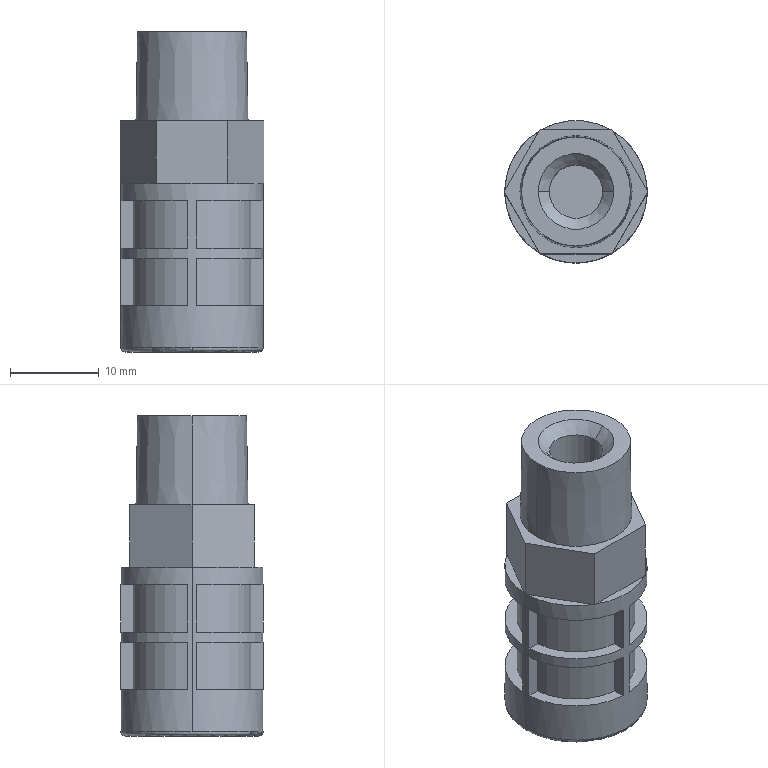Part | STEP file | CPS1-02-S silencer | 1 solid | 81 faces | box 16.166 x 16 x 36 mm | volume 5010 mm3 | plane 61 | cylinder 14 | cone 4 | torus 2 | commonest cylinder face diameters 13.3 x8 6 x4 16 x2